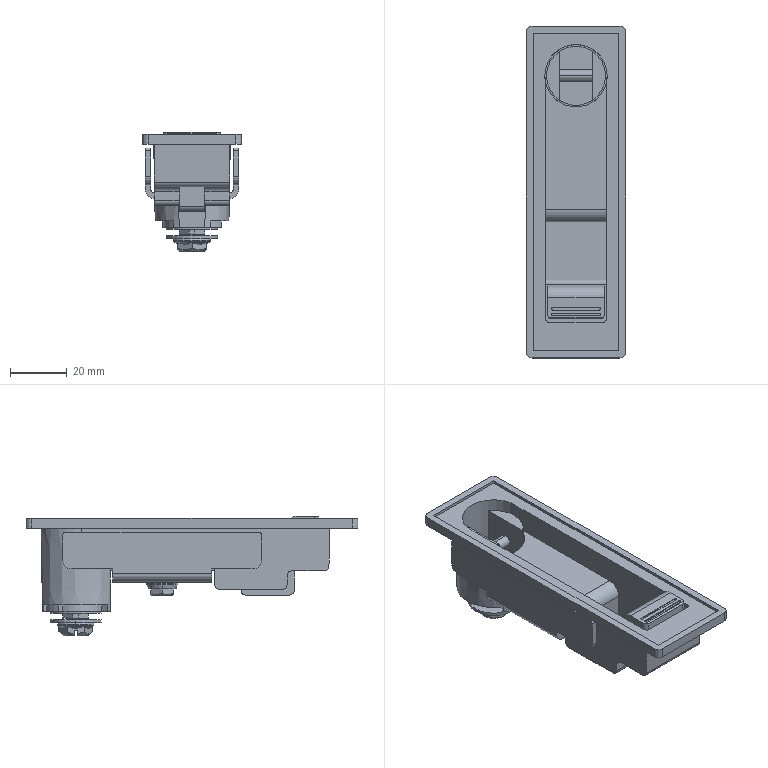Part | SolidWorks | features BaseBody 1 | 1 solid | 253 faces | box 35 x 117 x 42.2 mm | volume 38126 mm3 | plane 161 | cylinder 70 | cone 16 | torus 6 | commonest cylinder face diameters 3.4 x9 6 x8 0.8 x6 2 x6 3 x5 4 x4